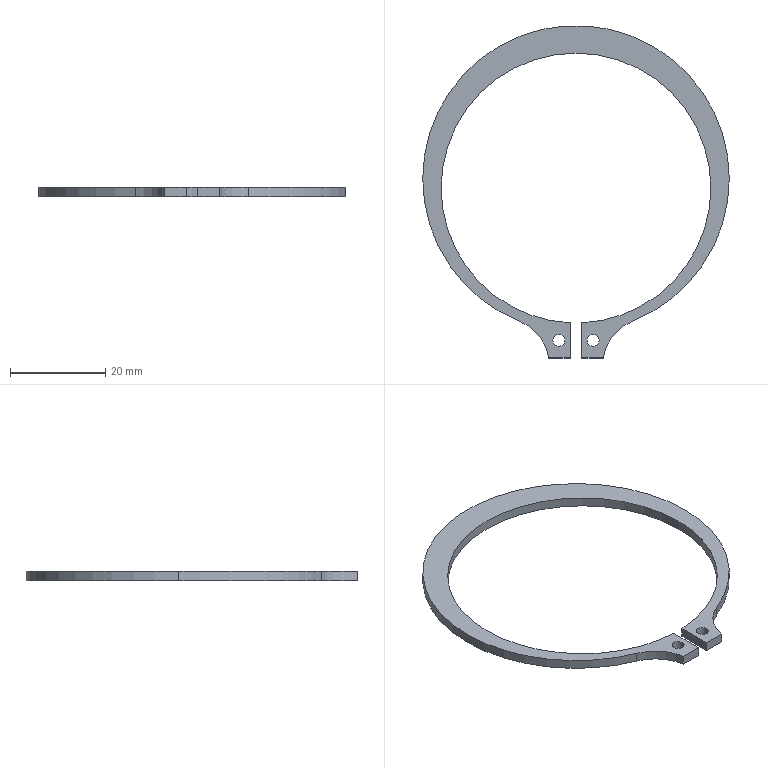Part | SolidWorks | features BaseBody 1 | 1 solid | 18 faces | box 64.433 x 69.873 x 2 mm | volume 1579 mm3 | cylinder 12 | plane 6 | commonest cylinder face diameters 2.5 x4 56.7 x3 64.433 x3 19.754 x2
STEP:
#1=CARTESIAN_POINT('',(4.858,-32.023,0.));
#2=VERTEX_POINT('',#1);
#3=CARTESIAN_POINT('',(2.358,-32.023,0.));
#4=VERTEX_POINT('',#3);
#5=CARTESIAN_POINT('',(3.608,-32.023,0.));
#6=DIRECTION('',(0.,0.,-1.));
#7=DIRECTION('',(-1.,0.,0.));
#8=AXIS2_PLACEMENT_3D('',#5,#6,#7);
#9=CIRCLE('',#8,1.25);
#10=EDGE_CURVE('',#2,#4,#9,.T.);
#11=ORIENTED_EDGE('',*,*,#10,.F.);
#12=CARTESIAN_POINT('',(4.858,-32.023,-2.));
#13=VERTEX_POINT('',#12);
#14=CARTESIAN_POINT('',(4.858,-32.023,0.));
#15=DIRECTION('',(0.,0.,-1.));
#16=VECTOR('',#15,1000.);
#17=LINE('',#14,#16);
#18=EDGE_CURVE('',#2,#13,#17,.T.);
#19=ORIENTED_EDGE('',*,*,#18,.T.);
#20=CARTESIAN_POINT('',(2.358,-32.023,-2.));
#21=VERTEX_POINT('',#20);
#22=CARTESIAN_POINT('',(3.608,-32.023,-2.));
#23=DIRECTION('',(0.,0.,-1.));
#24=DIRECTION('',(-1.,0.,0.));
#25=AXIS2_PLACEMENT_3D('',#22,#23,#24);
#26=CIRCLE('',#25,1.25);
#27=EDGE_CURVE('',#13,#21,#26,.T.);
#28=ORIENTED_EDGE('',*,*,#27,.T.);
#29=CARTESIAN_POINT('',(2.358,-32.023,0.));
#30=DIRECTION('',(0.,0.,-1.));
#31=VECTOR('',#30,1000.);
#32=LINE('',#29,#31);
#33=EDGE_CURVE('',#4,#21,#32,.T.);
#34=ORIENTED_EDGE('',*,*,#33,.F.);
#35=EDGE_LOOP('',(#11,#19,#28,#34));
#36=FACE_OUTER_BOUND('',#35,.T.);
#37=CARTESIAN_POINT('',(3.608,-32.023,0.));
#38=DIRECTION('',(0.,0.,-1.));
#39=DIRECTION('',(-1.,0.,0.));
#40=AXIS2_PLACEMENT_3D('',#37,#38,#39);
#41=CYLINDRICAL_SURFACE('',#40,1.25);
#42=ADVANCED_FACE('',(#36),#41,.F.);
#43=CARTESIAN_POINT('',(-2.358,-32.023,0.));
#44=VERTEX_POINT('',#43);
#45=CARTESIAN_POINT('',(-4.858,-32.023,0.));
#46=VERTEX_POINT('',#45);
#47=CARTESIAN_POINT('',(-3.608,-32.023,0.));
#48=DIRECTION('',(0.,0.,-1.));
#49=DIRECTION('',(-1.,0.,0.));
#50=AXIS2_PLACEMENT_3D('',#47,#48,#49);
#51=CIRCLE('',#50,1.25);
#52=EDGE_CURVE('',#44,#46,#51,.T.);
#53=ORIENTED_EDGE('',*,*,#52,.F.);
#54=CARTESIAN_POINT('',(-2.358,-32.023,-2.));
#55=VERTEX_POINT('',#54);
#56=CARTESIAN_POINT('',(-2.358,-32.023,0.));
#57=DIRECTION('',(0.,0.,-1.));
#58=VECTOR('',#57,1000.);
#59=LINE('',#56,#58);
#60=EDGE_CURVE('',#44,#55,#59,.T.);
#61=ORIENTED_EDGE('',*,*,#60,.T.);
#62=CARTESIAN_POINT('',(-4.858,-32.023,-2.));
#63=VERTEX_POINT('',#62);
#64=CARTESIAN_POINT('',(-3.608,-32.023,-2.));
#65=DIRECTION('',(0.,0.,-1.));
#66=DIRECTION('',(-1.,0.,0.));
#67=AXIS2_PLACEMENT_3D('',#64,#65,#66);
#68=CIRCLE('',#67,1.25);
#69=EDGE_CURVE('',#55,#63,#68,.T.);
#70=ORIENTED_EDGE('',*,*,#69,.T.);
#71=CARTESIAN_POINT('',(-4.858,-32.023,0.));
#72=DIRECTION('',(0.,0.,-1.));
#73=VECTOR('',#72,1000.);
#74=LINE('',#71,#73);
#75=EDGE_CURVE('',#46,#63,#74,.T.);
#76=ORIENTED_EDGE('',*,*,#75,.F.);
#77=EDGE_LOOP('',(#53,#61,#70,#76));
#78=FACE_OUTER_BOUND('',#77,.T.);
#79=CARTESIAN_POINT('',(-3.608,-32.023,0.));
#80=DIRECTION('',(0.,0.,-1.));
#81=DIRECTION('',(-1.,0.,0.));
#82=AXIS2_PLACEMENT_3D('',#79,#80,#81);
#83=CYLINDRICAL_SURFACE('',#82,1.25);
#84=ADVANCED_FACE('',(#78),#83,.F.);
#85=CARTESIAN_POINT('',(-32.217,1.933,0.));
#86=VERTEX_POINT('',#85);
#87=CARTESIAN_POINT('',(32.217,1.933,0.));
#88=VERTEX_POINT('',#87);
#89=CARTESIAN_POINT('',(0.,1.933,0.));
#90=DIRECTION('',(0.,0.,-1.));
#91=DIRECTION('',(-1.,0.,0.));
#92=AXIS2_PLACEMENT_3D('',#89,#90,#91);
#93=CIRCLE('',#92,32.217);
#94=EDGE_CURVE('',#86,#88,#93,.T.);
#95=ORIENTED_EDGE('',*,*,#94,.T.);
#96=CARTESIAN_POINT('',(32.217,1.933,-2.));
#97=VERTEX_POINT('',#96);
#98=CARTESIAN_POINT('',(32.217,1.933,0.));
#99=DIRECTION('',(0.,0.,-1.));
#100=VECTOR('',#99,1000.);
#101=LINE('',#98,#100);
#102=EDGE_CURVE('',#88,#97,#101,.T.);
#103=ORIENTED_EDGE('',*,*,#102,.T.);
#104=CARTESIAN_POINT('',(-32.217,1.933,-2.));
#105=VERTEX_POINT('',#104);
#106=CARTESIAN_POINT('',(0.,1.933,-2.));
#107=DIRECTION('',(0.,0.,1.));
#108=DIRECTION('',(-1.,0.,0.));
#109=AXIS2_PLACEMENT_3D('',#106,#107,#108);
#110=CIRCLE('',#109,32.217);
#111=EDGE_CURVE('',#97,#105,#110,.T.);
#112=ORIENTED_EDGE('',*,*,#111,.T.);
#113=CARTESIAN_POINT('',(-32.217,1.933,0.));
#114=DIRECTION('',(0.,0.,-1.));
#115=VECTOR('',#114,1000.);
#116=LINE('',#113,#115);
#117=EDGE_CURVE('',#86,#105,#116,.T.);
#118=ORIENTED_EDGE('',*,*,#117,.F.);
#119=EDGE_LOOP('',(#95,#103,#112,#118));
#120=FACE_OUTER_BOUND('',#119,.T.);
#121=CARTESIAN_POINT('',(0.,1.933,0.));
#122=DIRECTION('',(0.,0.,-1.));
#123=DIRECTION('',(-1.,0.,0.));
#124=AXIS2_PLACEMENT_3D('',#121,#122,#123);
#125=CYLINDRICAL_SURFACE('',#124,32.217);
#126=ADVANCED_FACE('',(#120),#125,.T.);
#127=CARTESIAN_POINT('',(-11.862,-28.02,0.));
#128=VERTEX_POINT('',#127);
#129=CARTESIAN_POINT('',(0.,1.933,0.));
#130=DIRECTION('',(0.,0.,-1.));
#131=DIRECTION('',(-1.,0.,0.));
#132=AXIS2_PLACEMENT_3D('',#129,#130,#131);
#133=CIRCLE('',#132,32.217);
#134=EDGE_CURVE('',#128,#86,#133,.T.);
#135=ORIENTED_EDGE('',*,*,#134,.T.);
#136=ORIENTED_EDGE('',*,*,#117,.T.);
#137=CARTESIAN_POINT('',(-11.862,-28.02,-2.));
#138=VERTEX_POINT('',#137);
#139=CARTESIAN_POINT('',(0.,1.933,-2.));
#140=DIRECTION('',(0.,0.,1.));
#141=DIRECTION('',(-1.,0.,0.));
#142=AXIS2_PLACEMENT_3D('',#139,#140,#141);
#143=CIRCLE('',#142,32.217);
#144=EDGE_CURVE('',#105,#138,#143,.T.);
#145=ORIENTED_EDGE('',*,*,#144,.T.);
#146=CARTESIAN_POINT('',(-11.862,-28.02,0.));
#147=DIRECTION('',(0.,0.,1.));
#148=VECTOR('',#147,1000.);
#149=LINE('',#146,#148);
#150=EDGE_CURVE('',#138,#128,#149,.T.);
#151=ORIENTED_EDGE('',*,*,#150,.T.);
#152=EDGE_LOOP('',(#135,#136,#145,#151));
#153=FACE_OUTER_BOUND('',#152,.T.);
#154=CARTESIAN_POINT('',(0.,1.933,0.));
#155=DIRECTION('',(0.,0.,-1.));
#156=DIRECTION('',(-1.,0.,0.));
#157=AXIS2_PLACEMENT_3D('',#154,#155,#156);
#158=CYLINDRICAL_SURFACE('',#157,32.217);
#159=ADVANCED_FACE('',(#153),#158,.T.);
#160=CARTESIAN_POINT('',(28.35,0.,0.));
#161=VERTEX_POINT('',#160);
#162=CARTESIAN_POINT('',(1.233,-28.323,0.));
#163=VERTEX_POINT('',#162);
#164=CARTESIAN_POINT('',(0.,0.,0.));
#165=DIRECTION('',(0.,0.,-1.));
#166=DIRECTION('',(-1.,0.,0.));
#167=AXIS2_PLACEMENT_3D('',#164,#165,#166);
#168=CIRCLE('',#167,28.35);
#169=EDGE_CURVE('',#161,#163,#168,.T.);
#170=ORIENTED_EDGE('',*,*,#169,.F.);
#171=CARTESIAN_POINT('',(28.35,0.,-2.));
#172=VERTEX_POINT('',#171);
#173=CARTESIAN_POINT('',(28.35,0.,0.));
#174=DIRECTION('',(0.,0.,-1.));
#175=VECTOR('',#174,1000.);
#176=LINE('',#173,#175);
#177=EDGE_CURVE('',#161,#172,#176,.T.);
#178=ORIENTED_EDGE('',*,*,#177,.T.);
#179=CARTESIAN_POINT('',(1.233,-28.323,-2.));
#180=VERTEX_POINT('',#179);
#181=CARTESIAN_POINT('',(0.,0.,-2.));
#182=DIRECTION('',(0.,0.,-1.));
#183=DIRECTION('',(-1.,0.,0.));
#184=AXIS2_PLACEMENT_3D('',#181,#182,#183);
#185=CIRCLE('',#184,28.35);
#186=EDGE_CURVE('',#172,#180,#185,.T.);
#187=ORIENTED_EDGE('',*,*,#186,.T.);
#188=CARTESIAN_POINT('',(1.233,-28.323,0.));
#189=DIRECTION('',(0.,0.,-1.));
#190=VECTOR('',#189,1000.);
#191=LINE('',#188,#190);
#192=EDGE_CURVE('',#163,#180,#191,.T.);
#193=ORIENTED_EDGE('',*,*,#192,.F.);
#194=EDGE_LOOP('',(#170,#178,#187,#193));
#195=FACE_OUTER_BOUND('',#194,.T.);
#196=CARTESIAN_POINT('',(0.,0.,0.));
#197=DIRECTION('',(0.,0.,-1.));
#198=DIRECTION('',(-1.,0.,0.));
#199=AXIS2_PLACEMENT_3D('',#196,#197,#198);
#200=CYLINDRICAL_SURFACE('',#199,28.35);
#201=ADVANCED_FACE('',(#195),#200,.F.);
#202=ORIENTED_EDGE('',*,*,#177,.F.);
#203=CARTESIAN_POINT('',(-28.35,0.,0.));
#204=VERTEX_POINT('',#203);
#205=CARTESIAN_POINT('',(0.,0.,0.));
#206=DIRECTION('',(0.,0.,-1.));
#207=DIRECTION('',(-1.,0.,0.));
#208=AXIS2_PLACEMENT_3D('',#205,#206,#207);
#209=CIRCLE('',#208,28.35);
#210=EDGE_CURVE('',#204,#161,#209,.T.);
#211=ORIENTED_EDGE('',*,*,#210,.F.);
#212=CARTESIAN_POINT('',(-28.35,0.,-2.));
#213=VERTEX_POINT('',#212);
#214=CARTESIAN_POINT('',(-28.35,0.,0.));
#215=DIRECTION('',(0.,0.,-1.));
#216=VECTOR('',#215,1000.);
#217=LINE('',#214,#216);
#218=EDGE_CURVE('',#204,#213,#217,.T.);
#219=ORIENTED_EDGE('',*,*,#218,.T.);
#220=CARTESIAN_POINT('',(0.,0.,-2.));
#221=DIRECTION('',(0.,0.,-1.));
#222=DIRECTION('',(-1.,0.,0.));
#223=AXIS2_PLACEMENT_3D('',#220,#221,#222);
#224=CIRCLE('',#223,28.35);
#225=EDGE_CURVE('',#213,#172,#224,.T.);
#226=ORIENTED_EDGE('',*,*,#225,.T.);
#227=EDGE_LOOP('',(#202,#211,#219,#226));
#228=FACE_OUTER_BOUND('',#227,.T.);
#229=CARTESIAN_POINT('',(0.,0.,0.));
#230=DIRECTION('',(0.,0.,-1.));
#231=DIRECTION('',(-1.,0.,0.));
#232=AXIS2_PLACEMENT_3D('',#229,#230,#231);
#233=CYLINDRICAL_SURFACE('',#232,28.35);
#234=ADVANCED_FACE('',(#228),#233,.F.);
#235=CARTESIAN_POINT('',(3.608,-32.023,-2.));
#236=DIRECTION('',(0.,0.,-1.));
#237=DIRECTION('',(-1.,0.,0.));
#238=AXIS2_PLACEMENT_3D('',#235,#236,#237);
#239=CIRCLE('',#238,1.25);
#240=EDGE_CURVE('',#21,#13,#239,.T.);
#241=ORIENTED_EDGE('',*,*,#240,.F.);
#242=ORIENTED_EDGE('',*,*,#27,.F.);
#243=EDGE_LOOP('',(#241,#242));
#244=FACE_BOUND('',#243,.T.);
#245=CARTESIAN_POINT('',(-3.608,-32.023,-2.));
#246=DIRECTION('',(0.,0.,-1.));
#247=DIRECTION('',(-1.,0.,0.));
#248=AXIS2_PLACEMENT_3D('',#245,#246,#247);
#249=CIRCLE('',#248,1.25);
#250=EDGE_CURVE('',#63,#55,#249,.T.);
#251=ORIENTED_EDGE('',*,*,#250,.F.);
#252=ORIENTED_EDGE('',*,*,#69,.F.);
#253=EDGE_LOOP('',(#251,#252));
#254=FACE_BOUND('',#253,.T.);
#255=CARTESIAN_POINT('',(-5.733,-35.723,-2.));
#256=VERTEX_POINT('',#255);
#257=CARTESIAN_POINT('',(-1.233,-35.723,-2.));
#258=VERTEX_POINT('',#257);
#259=CARTESIAN_POINT('',(0.,-35.723,-2.));
#260=DIRECTION('',(1.,0.,0.));
#261=VECTOR('',#260,1000.);
#262=LINE('',#259,#261);
#263=EDGE_CURVE('',#256,#258,#262,.T.);
#264=ORIENTED_EDGE('',*,*,#263,.F.);
#265=CARTESIAN_POINT('',(-15.499,-37.203,-2.));
#266=DIRECTION('',(0.,0.,-1.));
#267=DIRECTION('',(-1.,0.,0.));
#268=AXIS2_PLACEMENT_3D('',#265,#266,#267);
#269=CIRCLE('',#268,9.877);
#270=EDGE_CURVE('',#138,#256,#269,.T.);
#271=ORIENTED_EDGE('',*,*,#270,.F.);
#272=ORIENTED_EDGE('',*,*,#144,.F.);
#273=ORIENTED_EDGE('',*,*,#111,.F.);
#274=CARTESIAN_POINT('',(11.862,-28.02,-2.));
#275=VERTEX_POINT('',#274);
#276=CARTESIAN_POINT('',(0.,1.933,-2.));
#277=DIRECTION('',(0.,0.,1.));
#278=DIRECTION('',(-1.,0.,0.));
#279=AXIS2_PLACEMENT_3D('',#276,#277,#278);
#280=CIRCLE('',#279,32.217);
#281=EDGE_CURVE('',#275,#97,#280,.T.);
#282=ORIENTED_EDGE('',*,*,#281,.F.);
#283=CARTESIAN_POINT('',(5.733,-35.723,-2.));
#284=VERTEX_POINT('',#283);
#285=CARTESIAN_POINT('',(15.499,-37.203,-2.));
#286=DIRECTION('',(0.,0.,-1.));
#287=DIRECTION('',(-1.,0.,0.));
#288=AXIS2_PLACEMENT_3D('',#285,#286,#287);
#289=CIRCLE('',#288,9.877);
#290=EDGE_CURVE('',#284,#275,#289,.T.);
#291=ORIENTED_EDGE('',*,*,#290,.F.);
#292=CARTESIAN_POINT('',(1.233,-35.723,-2.));
#293=VERTEX_POINT('',#292);
#294=CARTESIAN_POINT('',(0.,-35.723,-2.));
#295=DIRECTION('',(1.,0.,0.));
#296=VECTOR('',#295,1000.);
#297=LINE('',#294,#296);
#298=EDGE_CURVE('',#293,#284,#297,.T.);
#299=ORIENTED_EDGE('',*,*,#298,.F.);
#300=CARTESIAN_POINT('',(1.233,-3.256,-2.));
#301=DIRECTION('',(0.,-1.,0.));
#302=VECTOR('',#301,1000.);
#303=LINE('',#300,#302);
#304=EDGE_CURVE('',#180,#293,#303,.T.);
#305=ORIENTED_EDGE('',*,*,#304,.F.);
#306=ORIENTED_EDGE('',*,*,#186,.F.);
#307=ORIENTED_EDGE('',*,*,#225,.F.);
#308=CARTESIAN_POINT('',(-1.233,-28.323,-2.));
#309=VERTEX_POINT('',#308);
#310=CARTESIAN_POINT('',(0.,0.,-2.));
#311=DIRECTION('',(0.,0.,-1.));
#312=DIRECTION('',(-1.,0.,0.));
#313=AXIS2_PLACEMENT_3D('',#310,#311,#312);
#314=CIRCLE('',#313,28.35);
#315=EDGE_CURVE('',#309,#213,#314,.T.);
#316=ORIENTED_EDGE('',*,*,#315,.F.);
#317=CARTESIAN_POINT('',(-1.233,-3.256,-2.));
#318=DIRECTION('',(0.,1.,0.));
#319=VECTOR('',#318,1000.);
#320=LINE('',#317,#319);
#321=EDGE_CURVE('',#258,#309,#320,.T.);
#322=ORIENTED_EDGE('',*,*,#321,.F.);
#323=EDGE_LOOP('',(#264,#271,#272,#273,#282,#291,#299,#305,#306,#307,#316,#322));
#324=FACE_OUTER_BOUND('',#323,.T.);
#325=CARTESIAN_POINT('',(0.,-3.256,-2.));
#326=DIRECTION('',(0.,0.,1.));
#327=DIRECTION('',(1.,0.,0.));
#328=AXIS2_PLACEMENT_3D('',#325,#326,#327);
#329=PLANE('',#328);
#330=ADVANCED_FACE('',(#244,#254,#324),#329,.F.);
#331=ORIENTED_EDGE('',*,*,#18,.F.);
#332=CARTESIAN_POINT('',(3.608,-32.023,0.));
#333=DIRECTION('',(0.,0.,-1.));
#334=DIRECTION('',(-1.,0.,0.));
#335=AXIS2_PLACEMENT_3D('',#332,#333,#334);
#336=CIRCLE('',#335,1.25);
#337=EDGE_CURVE('',#4,#2,#336,.T.);
#338=ORIENTED_EDGE('',*,*,#337,.F.);
#339=ORIENTED_EDGE('',*,*,#33,.T.);
#340=ORIENTED_EDGE('',*,*,#240,.T.);
#341=EDGE_LOOP('',(#331,#338,#339,#340));
#342=FACE_OUTER_BOUND('',#341,.T.);
#343=CARTESIAN_POINT('',(3.608,-32.023,0.));
#344=DIRECTION('',(0.,0.,-1.));
#345=DIRECTION('',(-1.,0.,0.));
#346=AXIS2_PLACEMENT_3D('',#343,#344,#345);
#347=CYLINDRICAL_SURFACE('',#346,1.25);
#348=ADVANCED_FACE('',(#342),#347,.F.);
#349=ORIENTED_EDGE('',*,*,#60,.F.);
#350=CARTESIAN_POINT('',(-3.608,-32.023,0.));
#351=DIRECTION('',(0.,0.,-1.));
#352=DIRECTION('',(-1.,0.,0.));
#353=AXIS2_PLACEMENT_3D('',#350,#351,#352);
#354=CIRCLE('',#353,1.25);
#355=EDGE_CURVE('',#46,#44,#354,.T.);
#356=ORIENTED_EDGE('',*,*,#355,.F.);
#357=ORIENTED_EDGE('',*,*,#75,.T.);
#358=ORIENTED_EDGE('',*,*,#250,.T.);
#359=EDGE_LOOP('',(#349,#356,#357,#358));
#360=FACE_OUTER_BOUND('',#359,.T.);
#361=CARTESIAN_POINT('',(-3.608,-32.023,0.));
#362=DIRECTION('',(0.,0.,-1.));
#363=DIRECTION('',(-1.,0.,0.));
#364=AXIS2_PLACEMENT_3D('',#361,#362,#363);
#365=CYLINDRICAL_SURFACE('',#364,1.25);
#366=ADVANCED_FACE('',(#360),#365,.F.);
#367=CARTESIAN_POINT('',(-1.233,-28.323,0.));
#368=VERTEX_POINT('',#367);
#369=CARTESIAN_POINT('',(-1.233,-35.723,0.));
#370=VERTEX_POINT('',#369);
#371=CARTESIAN_POINT('',(-1.233,-35.723,0.));
#372=DIRECTION('',(0.,-1.,0.));
#373=VECTOR('',#372,1000.);
#374=LINE('',#371,#373);
#375=EDGE_CURVE('',#368,#370,#374,.T.);
#376=ORIENTED_EDGE('',*,*,#375,.T.);
#377=CARTESIAN_POINT('',(-1.233,-35.723,0.));
#378=DIRECTION('',(0.,0.,-1.));
#379=VECTOR('',#378,1000.);
#380=LINE('',#377,#379);
#381=EDGE_CURVE('',#370,#258,#380,.T.);
#382=ORIENTED_EDGE('',*,*,#381,.T.);
#383=ORIENTED_EDGE('',*,*,#321,.T.);
#384=CARTESIAN_POINT('',(-1.233,-28.323,0.));
#385=DIRECTION('',(0.,0.,1.));
#386=VECTOR('',#385,1000.);
#387=LINE('',#384,#386);
#388=EDGE_CURVE('',#309,#368,#387,.T.);
#389=ORIENTED_EDGE('',*,*,#388,.T.);
#390=EDGE_LOOP('',(#376,#382,#383,#389));
#391=FACE_OUTER_BOUND('',#390,.T.);
#392=CARTESIAN_POINT('',(-1.233,-35.723,0.));
#393=DIRECTION('',(1.,0.,0.));
#394=DIRECTION('',(0.,1.,0.));
#395=AXIS2_PLACEMENT_3D('',#392,#393,#394);
#396=PLANE('',#395);
#397=ADVANCED_FACE('',(#391),#396,.T.);
#398=CARTESIAN_POINT('',(-5.733,-35.723,0.));
#399=VERTEX_POINT('',#398);
#400=CARTESIAN_POINT('',(-5.733,-35.723,0.));
#401=DIRECTION('',(-1.,0.,0.));
#402=VECTOR('',#401,1000.);
#403=LINE('',#400,#402);
#404=EDGE_CURVE('',#370,#399,#403,.T.);
#405=ORIENTED_EDGE('',*,*,#404,.T.);
#406=CARTESIAN_POINT('',(-5.733,-35.723,0.));
#407=DIRECTION('',(0.,0.,-1.));
#408=VECTOR('',#407,1000.);
#409=LINE('',#406,#408);
#410=EDGE_CURVE('',#399,#256,#409,.T.);
#411=ORIENTED_EDGE('',*,*,#410,.T.);
#412=ORIENTED_EDGE('',*,*,#263,.T.);
#413=ORIENTED_EDGE('',*,*,#381,.F.);
#414=EDGE_LOOP('',(#405,#411,#412,#413));
#415=FACE_OUTER_BOUND('',#414,.T.);
#416=CARTESIAN_POINT('',(-5.733,-35.723,0.));
#417=DIRECTION('',(0.,-1.,0.));
#418=DIRECTION('',(1.,0.,0.));
#419=AXIS2_PLACEMENT_3D('',#416,#417,#418);
#420=PLANE('',#419);
#421=ADVANCED_FACE('',(#415),#420,.T.);
#422=ORIENTED_EDGE('',*,*,#410,.F.);
#423=CARTESIAN_POINT('',(-15.499,-37.203,0.));
#424=DIRECTION('',(0.,0.,-1.));
#425=DIRECTION('',(-1.,0.,0.));
#426=AXIS2_PLACEMENT_3D('',#423,#424,#425);
#427=CIRCLE('',#426,9.877);
#428=EDGE_CURVE('',#128,#399,#427,.T.);
#429=ORIENTED_EDGE('',*,*,#428,.F.);
#430=ORIENTED_EDGE('',*,*,#150,.F.);
#431=ORIENTED_EDGE('',*,*,#270,.T.);
#432=EDGE_LOOP('',(#422,#429,#430,#431));
#433=FACE_OUTER_BOUND('',#432,.T.);
#434=CARTESIAN_POINT('',(-15.499,-37.203,0.));
#435=DIRECTION('',(0.,0.,-1.));
#436=DIRECTION('',(-1.,0.,0.));
#437=AXIS2_PLACEMENT_3D('',#434,#435,#436);
#438=CYLINDRICAL_SURFACE('',#437,9.877);
#439=ADVANCED_FACE('',(#433),#438,.F.);
#440=ORIENTED_EDGE('',*,*,#102,.F.);
#441=CARTESIAN_POINT('',(11.862,-28.02,0.));
#442=VERTEX_POINT('',#441);
#443=CARTESIAN_POINT('',(0.,1.933,0.));
#444=DIRECTION('',(0.,0.,-1.));
#445=DIRECTION('',(-1.,0.,0.));
#446=AXIS2_PLACEMENT_3D('',#443,#444,#445);
#447=CIRCLE('',#446,32.217);
#448=EDGE_CURVE('',#88,#442,#447,.T.);
#449=ORIENTED_EDGE('',*,*,#448,.T.);
#450=CARTESIAN_POINT('',(11.862,-28.02,0.));
#451=DIRECTION('',(0.,0.,-1.));
#452=VECTOR('',#451,1000.);
#453=LINE('',#450,#452);
#454=EDGE_CURVE('',#442,#275,#453,.T.);
#455=ORIENTED_EDGE('',*,*,#454,.T.);
#456=ORIENTED_EDGE('',*,*,#281,.T.);
#457=EDGE_LOOP('',(#440,#449,#455,#456));
#458=FACE_OUTER_BOUND('',#457,.T.);
#459=CARTESIAN_POINT('',(0.,1.933,0.));
#460=DIRECTION('',(0.,0.,-1.));
#461=DIRECTION('',(-1.,0.,0.));
#462=AXIS2_PLACEMENT_3D('',#459,#460,#461);
#463=CYLINDRICAL_SURFACE('',#462,32.217);
#464=ADVANCED_FACE('',(#458),#463,.T.);
#465=ORIENTED_EDGE('',*,*,#454,.F.);
#466=CARTESIAN_POINT('',(5.733,-35.723,0.));
#467=VERTEX_POINT('',#466);
#468=CARTESIAN_POINT('',(15.499,-37.203,0.));
#469=DIRECTION('',(0.,0.,-1.));
#470=DIRECTION('',(-1.,0.,0.));
#471=AXIS2_PLACEMENT_3D('',#468,#469,#470);
#472=CIRCLE('',#471,9.877);
#473=EDGE_CURVE('',#467,#442,#472,.T.);
#474=ORIENTED_EDGE('',*,*,#473,.F.);
#475=CARTESIAN_POINT('',(5.733,-35.723,0.));
#476=DIRECTION('',(0.,0.,1.));
#477=VECTOR('',#476,1000.);
#478=LINE('',#475,#477);
#479=EDGE_CURVE('',#284,#467,#478,.T.);
#480=ORIENTED_EDGE('',*,*,#479,.F.);
#481=ORIENTED_EDGE('',*,*,#290,.T.);
#482=EDGE_LOOP('',(#465,#474,#480,#481));
#483=FACE_OUTER_BOUND('',#482,.T.);
#484=CARTESIAN_POINT('',(15.499,-37.203,0.));
#485=DIRECTION('',(0.,0.,-1.));
#486=DIRECTION('',(-1.,0.,0.));
#487=AXIS2_PLACEMENT_3D('',#484,#485,#486);
#488=CYLINDRICAL_SURFACE('',#487,9.877);
#489=ADVANCED_FACE('',(#483),#488,.F.);
#490=CARTESIAN_POINT('',(1.233,-35.723,0.));
#491=VERTEX_POINT('',#490);
#492=CARTESIAN_POINT('',(1.233,-35.723,0.));
#493=DIRECTION('',(-1.,0.,0.));
#494=VECTOR('',#493,1000.);
#495=LINE('',#492,#494);
#496=EDGE_CURVE('',#467,#491,#495,.T.);
#497=ORIENTED_EDGE('',*,*,#496,.T.);
#498=CARTESIAN_POINT('',(1.233,-35.723,0.));
#499=DIRECTION('',(0.,0.,-1.));
#500=VECTOR('',#499,1000.);
#501=LINE('',#498,#500);
#502=EDGE_CURVE('',#491,#293,#501,.T.);
#503=ORIENTED_EDGE('',*,*,#502,.T.);
#504=ORIENTED_EDGE('',*,*,#298,.T.);
#505=ORIENTED_EDGE('',*,*,#479,.T.);
#506=EDGE_LOOP('',(#497,#503,#504,#505));
#507=FACE_OUTER_BOUND('',#506,.T.);
#508=CARTESIAN_POINT('',(1.233,-35.723,0.));
#509=DIRECTION('',(0.,-1.,0.));
#510=DIRECTION('',(1.,0.,0.));
#511=AXIS2_PLACEMENT_3D('',#508,#509,#510);
#512=PLANE('',#511);
#513=ADVANCED_FACE('',(#507),#512,.T.);
#514=CARTESIAN_POINT('',(1.233,-28.323,0.));
#515=DIRECTION('',(0.,1.,0.));
#516=VECTOR('',#515,1000.);
#517=LINE('',#514,#516);
#518=EDGE_CURVE('',#491,#163,#517,.T.);
#519=ORIENTED_EDGE('',*,*,#518,.T.);
#520=ORIENTED_EDGE('',*,*,#192,.T.);
#521=ORIENTED_EDGE('',*,*,#304,.T.);
#522=ORIENTED_EDGE('',*,*,#502,.F.);
#523=EDGE_LOOP('',(#519,#520,#521,#522));
#524=FACE_OUTER_BOUND('',#523,.T.);
#525=CARTESIAN_POINT('',(1.233,-28.323,0.));
#526=DIRECTION('',(-1.,0.,0.));
#527=DIRECTION('',(0.,-1.,0.));
#528=AXIS2_PLACEMENT_3D('',#525,#526,#527);
#529=PLANE('',#528);
#530=ADVANCED_FACE('',(#524),#529,.T.);
#531=ORIENTED_EDGE('',*,*,#218,.F.);
#532=CARTESIAN_POINT('',(0.,0.,0.));
#533=DIRECTION('',(0.,0.,-1.));
#534=DIRECTION('',(-1.,0.,0.));
#535=AXIS2_PLACEMENT_3D('',#532,#533,#534);
#536=CIRCLE('',#535,28.35);
#537=EDGE_CURVE('',#368,#204,#536,.T.);
#538=ORIENTED_EDGE('',*,*,#537,.F.);
#539=ORIENTED_EDGE('',*,*,#388,.F.);
#540=ORIENTED_EDGE('',*,*,#315,.T.);
#541=EDGE_LOOP('',(#531,#538,#539,#540));
#542=FACE_OUTER_BOUND('',#541,.T.);
#543=CARTESIAN_POINT('',(0.,0.,0.));
#544=DIRECTION('',(0.,0.,-1.));
#545=DIRECTION('',(-1.,0.,0.));
#546=AXIS2_PLACEMENT_3D('',#543,#544,#545);
#547=CYLINDRICAL_SURFACE('',#546,28.35);
#548=ADVANCED_FACE('',(#542),#547,.F.);
#549=ORIENTED_EDGE('',*,*,#337,.T.);
#550=ORIENTED_EDGE('',*,*,#10,.T.);
#551=EDGE_LOOP('',(#549,#550));
#552=FACE_BOUND('',#551,.T.);
#553=ORIENTED_EDGE('',*,*,#355,.T.);
#554=ORIENTED_EDGE('',*,*,#52,.T.);
#555=EDGE_LOOP('',(#553,#554));
#556=FACE_BOUND('',#555,.T.);
#557=ORIENTED_EDGE('',*,*,#134,.F.);
#558=ORIENTED_EDGE('',*,*,#428,.T.);
#559=ORIENTED_EDGE('',*,*,#404,.F.);
#560=ORIENTED_EDGE('',*,*,#375,.F.);
#561=ORIENTED_EDGE('',*,*,#537,.T.);
#562=ORIENTED_EDGE('',*,*,#210,.T.);
#563=ORIENTED_EDGE('',*,*,#169,.T.);
#564=ORIENTED_EDGE('',*,*,#518,.F.);
#565=ORIENTED_EDGE('',*,*,#496,.F.);
#566=ORIENTED_EDGE('',*,*,#473,.T.);
#567=ORIENTED_EDGE('',*,*,#448,.F.);
#568=ORIENTED_EDGE('',*,*,#94,.F.);
#569=EDGE_LOOP('',(#557,#558,#559,#560,#561,#562,#563,#564,#565,#566,#567,#568));
#570=FACE_OUTER_BOUND('',#569,.T.);
#571=CARTESIAN_POINT('',(0.,-3.256,0.));
#572=DIRECTION('',(0.,0.,1.));
#573=DIRECTION('',(1.,0.,0.));
#574=AXIS2_PLACEMENT_3D('',#571,#572,#573);
#575=PLANE('',#574);
#576=ADVANCED_FACE('',(#552,#556,#570),#575,.T.);
#577=CLOSED_SHELL('',(#42,#84,#126,#159,#201,#234,#330,#348,#366,#397,#421,#439,#464,#489,#513,#530,#548,#576));
#578=MANIFOLD_SOLID_BREP('',#577);
#579=CARTESIAN_POINT('',(0.,0.,0.));
#580=DIRECTION('',(0.,0.,1.));
#581=DIRECTION('',(1.,0.,0.));
#582=AXIS2_PLACEMENT_3D('',#579,#580,#581);
#583=(LENGTH_UNIT()NAMED_UNIT(*)SI_UNIT(.MILLI.,.METRE.));
#584=UNCERTAINTY_MEASURE_WITH_UNIT(LENGTH_MEASURE(0.00001),#583,'','');
#585=(NAMED_UNIT(*)PLANE_ANGLE_UNIT()SI_UNIT($,.RADIAN.));
#586=(NAMED_UNIT(*)SI_UNIT($,.STERADIAN.)SOLID_ANGLE_UNIT());
#587=(GEOMETRIC_REPRESENTATION_CONTEXT(3)GLOBAL_UNCERTAINTY_ASSIGNED_CONTEXT((#584))GLOBAL_UNIT_ASSIGNED_CONTEXT((#583,#585,#586))REPRESENTATION_CONTEXT('',''));
#588=ADVANCED_BREP_SHAPE_REPRESENTATION('',(#578,#582),#587);